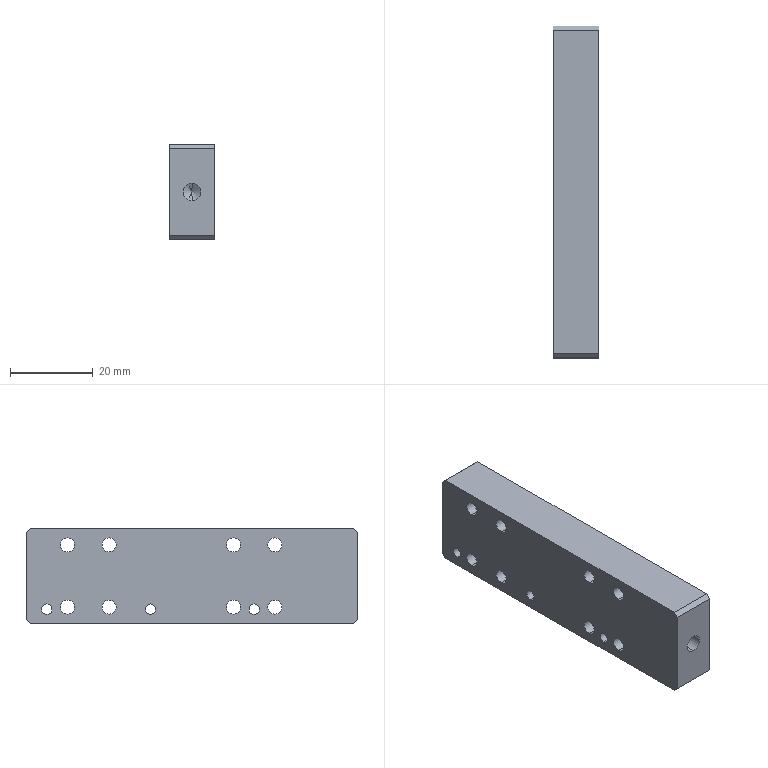Part | SolidWorks | features HoleWzd 3, Chamfer 1, Extrusion 1, ICE 1 | 1 solid | 65 faces | box 11 x 80 x 23 mm | volume 16527 mm3 | cylinder 41 | plane 22 | cone 2 | commonest cylinder face diameters 3.4 x16 6 x16 2.5 x6 4.2 x2 1 x1